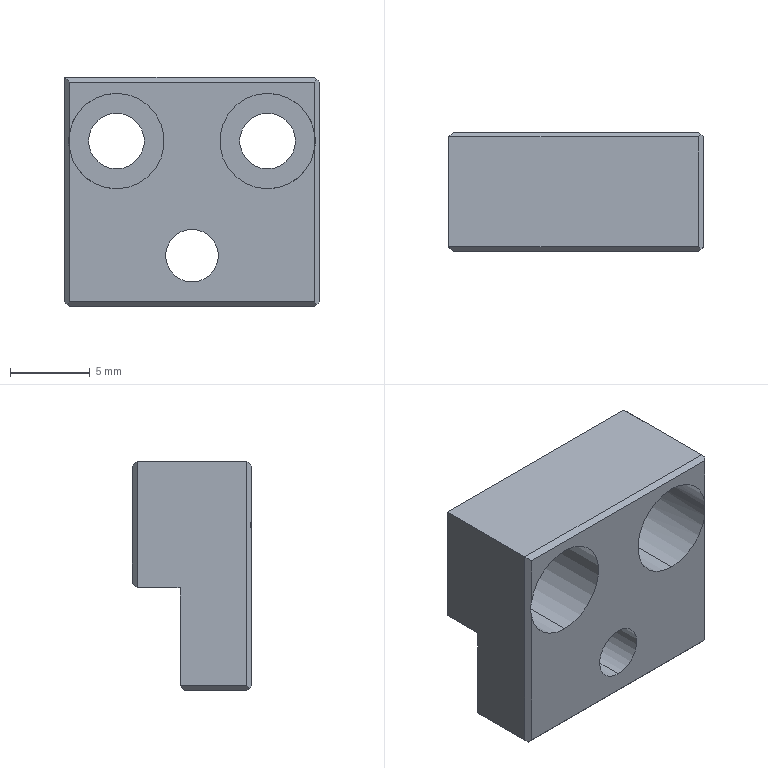Part | NX | 1 solid | 32 faces | box 16 x 7.5 x 14.4 mm | volume 1061 mm3 | plane 22 | cylinder 10 | commonest cylinder face diameters 3.5 x4 6 x4 3.3 x2
STEP:
#1=CARTESIAN_POINT('',(16.39,-63.429,11.453));
#2=VERTEX_POINT('',#1);
#3=CARTESIAN_POINT('',(0.3897,-63.429,11.453));
#4=VERTEX_POINT('',#3);
#5=CARTESIAN_POINT('',(8.39,-63.429,11.453));
#6=DIRECTION('',(-1.,0.,0.));
#7=VECTOR('',#6,1000.);
#8=LINE('',#5,#7);
#9=EDGE_CURVE('',#2,#4,#8,.T.);
#10=ORIENTED_EDGE('',*,*,#9,.F.);
#11=CARTESIAN_POINT('',(16.39,-66.129,11.453));
#12=VERTEX_POINT('',#11);
#13=CARTESIAN_POINT('',(16.39,-59.69,11.453));
#14=DIRECTION('',(0.,1.,0.));
#15=VECTOR('',#14,1000.);
#16=LINE('',#13,#15);
#17=EDGE_CURVE('',#12,#2,#16,.T.);
#18=ORIENTED_EDGE('',*,*,#17,.F.);
#19=CARTESIAN_POINT('',(0.3897,-66.129,11.453));
#20=VERTEX_POINT('',#19);
#21=CARTESIAN_POINT('',(13.89,-66.129,11.453));
#22=DIRECTION('',(-1.,0.,0.));
#23=VECTOR('',#22,1000.);
#24=LINE('',#21,#23);
#25=EDGE_CURVE('',#12,#20,#24,.T.);
#26=ORIENTED_EDGE('',*,*,#25,.T.);
#27=CARTESIAN_POINT('',(0.3897,-59.69,11.453));
#28=DIRECTION('',(0.,1.,0.));
#29=VECTOR('',#28,1000.);
#30=LINE('',#27,#29);
#31=EDGE_CURVE('',#20,#4,#30,.T.);
#32=ORIENTED_EDGE('',*,*,#31,.T.);
#33=EDGE_LOOP('',(#10,#18,#26,#32));
#34=FACE_BOUND('',#33,.T.);
#35=CARTESIAN_POINT('',(13.89,-66.629,11.453));
#36=DIRECTION('',(0.,0.,-1.));
#37=DIRECTION('',(0.,-1.,0.));
#38=AXIS2_PLACEMENT_3D('',#35,#36,#37);
#39=PLANE('',#38);
#40=ADVANCED_FACE('',(#34),#39,.T.);
#41=CARTESIAN_POINT('',(16.39,-66.129,5.303));
#42=VERTEX_POINT('',#41);
#43=CARTESIAN_POINT('',(0.3897,-66.129,5.303));
#44=VERTEX_POINT('',#43);
#45=CARTESIAN_POINT('',(8.39,-66.129,5.303));
#46=DIRECTION('',(-1.,0.,0.));
#47=VECTOR('',#46,1000.);
#48=LINE('',#45,#47);
#49=EDGE_CURVE('',#42,#44,#48,.T.);
#50=ORIENTED_EDGE('',*,*,#49,.T.);
#51=CARTESIAN_POINT('',(0.3897,-66.129,11.106));
#52=DIRECTION('',(0.,0.,-1.));
#53=VECTOR('',#52,1000.);
#54=LINE('',#51,#53);
#55=EDGE_CURVE('',#20,#44,#54,.T.);
#56=ORIENTED_EDGE('',*,*,#55,.F.);
#57=ORIENTED_EDGE('',*,*,#25,.F.);
#58=CARTESIAN_POINT('',(16.39,-66.129,11.106));
#59=DIRECTION('',(0.,0.,-1.));
#60=VECTOR('',#59,1000.);
#61=LINE('',#58,#60);
#62=EDGE_CURVE('',#12,#42,#61,.T.);
#63=ORIENTED_EDGE('',*,*,#62,.T.);
#64=EDGE_LOOP('',(#50,#56,#57,#63));
#65=FACE_BOUND('',#64,.T.);
#66=CARTESIAN_POINT('',(8.39,-66.129,6.553));
#67=VERTEX_POINT('',#66);
#68=CARTESIAN_POINT('',(8.39,-66.129,9.853));
#69=VERTEX_POINT('',#68);
#70=CARTESIAN_POINT('',(8.39,-66.129,8.203));
#71=DIRECTION('',(0.,-1.,0.));
#72=DIRECTION('',(0.,0.,1.));
#73=AXIS2_PLACEMENT_3D('',#70,#71,#72);
#74=CIRCLE('',#73,1.65);
#75=EDGE_CURVE('',#67,#69,#74,.T.);
#76=ORIENTED_EDGE('',*,*,#75,.T.);
#77=CARTESIAN_POINT('',(8.39,-66.129,8.203));
#78=DIRECTION('',(0.,-1.,0.));
#79=DIRECTION('',(0.,0.,1.));
#80=AXIS2_PLACEMENT_3D('',#77,#78,#79);
#81=CIRCLE('',#80,1.65);
#82=EDGE_CURVE('',#69,#67,#81,.T.);
#83=ORIENTED_EDGE('',*,*,#82,.T.);
#84=EDGE_LOOP('',(#76,#83));
#85=FACE_BOUND('',#84,.T.);
#86=CARTESIAN_POINT('',(13.89,-66.129,5.503));
#87=DIRECTION('',(0.,1.,0.));
#88=DIRECTION('',(1.,0.,0.));
#89=AXIS2_PLACEMENT_3D('',#86,#87,#88);
#90=PLANE('',#89);
#91=ADVANCED_FACE('',(#65,#85),#90,.T.);
#92=CARTESIAN_POINT('',(0.6897,-70.329,5.003));
#93=VERTEX_POINT('',#92);
#94=CARTESIAN_POINT('',(16.09,-70.329,5.003));
#95=VERTEX_POINT('',#94);
#96=CARTESIAN_POINT('',(8.39,-70.329,5.003));
#97=DIRECTION('',(1.,0.,0.));
#98=VECTOR('',#97,1000.);
#99=LINE('',#96,#98);
#100=EDGE_CURVE('',#93,#95,#99,.T.);
#101=ORIENTED_EDGE('',*,*,#100,.F.);
#102=CARTESIAN_POINT('',(0.6897,-66.429,5.003));
#103=VERTEX_POINT('',#102);
#104=CARTESIAN_POINT('',(0.6897,-68.379,5.003));
#105=DIRECTION('',(0.,-1.,0.));
#106=VECTOR('',#105,1000.);
#107=LINE('',#104,#106);
#108=EDGE_CURVE('',#103,#93,#107,.T.);
#109=ORIENTED_EDGE('',*,*,#108,.F.);
#110=CARTESIAN_POINT('',(16.09,-66.429,5.003));
#111=VERTEX_POINT('',#110);
#112=CARTESIAN_POINT('',(8.39,-66.429,5.003));
#113=DIRECTION('',(-1.,0.,0.));
#114=VECTOR('',#113,1000.);
#115=LINE('',#112,#114);
#116=EDGE_CURVE('',#111,#103,#115,.T.);
#117=ORIENTED_EDGE('',*,*,#116,.F.);
#118=CARTESIAN_POINT('',(16.09,-68.379,5.003));
#119=DIRECTION('',(0.,-1.,0.));
#120=VECTOR('',#119,1000.);
#121=LINE('',#118,#120);
#122=EDGE_CURVE('',#111,#95,#121,.T.);
#123=ORIENTED_EDGE('',*,*,#122,.T.);
#124=EDGE_LOOP('',(#101,#109,#117,#123));
#125=FACE_BOUND('',#124,.T.);
#126=CARTESIAN_POINT('',(13.89,-70.329,5.003));
#127=DIRECTION('',(0.,0.,-1.));
#128=DIRECTION('',(0.,-1.,0.));
#129=AXIS2_PLACEMENT_3D('',#126,#127,#128);
#130=PLANE('',#129);
#131=ADVANCED_FACE('',(#125),#130,.T.);
#132=CARTESIAN_POINT('',(16.09,-70.629,19.103));
#133=VERTEX_POINT('',#132);
#134=CARTESIAN_POINT('',(0.6897,-70.629,19.103));
#135=VERTEX_POINT('',#134);
#136=CARTESIAN_POINT('',(8.39,-70.629,19.103));
#137=DIRECTION('',(-1.,0.,0.));
#138=VECTOR('',#137,1000.);
#139=LINE('',#136,#138);
#140=EDGE_CURVE('',#133,#135,#139,.T.);
#141=ORIENTED_EDGE('',*,*,#140,.T.);
#142=CARTESIAN_POINT('',(0.6897,-70.629,15.949));
#143=VERTEX_POINT('',#142);
#144=CARTESIAN_POINT('',(0.6897,-70.629,11.106));
#145=DIRECTION('',(0.,0.,-1.));
#146=VECTOR('',#145,1000.);
#147=LINE('',#144,#146);
#148=EDGE_CURVE('',#135,#143,#147,.T.);
#149=ORIENTED_EDGE('',*,*,#148,.T.);
#150=CARTESIAN_POINT('',(3.64,-70.629,18.403));
#151=VERTEX_POINT('',#150);
#152=CARTESIAN_POINT('',(3.64,-70.629,15.403));
#153=DIRECTION('',(0.,-1.,0.));
#154=DIRECTION('',(0.,0.,1.));
#155=AXIS2_PLACEMENT_3D('',#152,#153,#154);
#156=CIRCLE('',#155,3.);
#157=EDGE_CURVE('',#151,#143,#156,.T.);
#158=ORIENTED_EDGE('',*,*,#157,.F.);
#159=CARTESIAN_POINT('',(3.64,-70.629,12.403));
#160=VERTEX_POINT('',#159);
#161=CARTESIAN_POINT('',(3.64,-70.629,15.403));
#162=DIRECTION('',(0.,-1.,0.));
#163=DIRECTION('',(0.,0.,1.));
#164=AXIS2_PLACEMENT_3D('',#161,#162,#163);
#165=CIRCLE('',#164,3.);
#166=EDGE_CURVE('',#160,#151,#165,.T.);
#167=ORIENTED_EDGE('',*,*,#166,.F.);
#168=CARTESIAN_POINT('',(0.6897,-70.629,14.858));
#169=VERTEX_POINT('',#168);
#170=CARTESIAN_POINT('',(3.64,-70.629,15.403));
#171=DIRECTION('',(0.,-1.,0.));
#172=DIRECTION('',(0.,0.,1.));
#173=AXIS2_PLACEMENT_3D('',#170,#171,#172);
#174=CIRCLE('',#173,3.);
#175=EDGE_CURVE('',#169,#160,#174,.T.);
#176=ORIENTED_EDGE('',*,*,#175,.F.);
#177=CARTESIAN_POINT('',(0.6897,-70.629,5.303));
#178=VERTEX_POINT('',#177);
#179=CARTESIAN_POINT('',(0.6897,-70.629,11.106));
#180=DIRECTION('',(0.,0.,-1.));
#181=VECTOR('',#180,1000.);
#182=LINE('',#179,#181);
#183=EDGE_CURVE('',#169,#178,#182,.T.);
#184=ORIENTED_EDGE('',*,*,#183,.T.);
#185=CARTESIAN_POINT('',(16.09,-70.629,5.303));
#186=VERTEX_POINT('',#185);
#187=CARTESIAN_POINT('',(8.39,-70.629,5.303));
#188=DIRECTION('',(1.,0.,0.));
#189=VECTOR('',#188,1000.);
#190=LINE('',#187,#189);
#191=EDGE_CURVE('',#178,#186,#190,.T.);
#192=ORIENTED_EDGE('',*,*,#191,.T.);
#193=CARTESIAN_POINT('',(16.09,-70.629,14.858));
#194=VERTEX_POINT('',#193);
#195=CARTESIAN_POINT('',(16.09,-70.629,11.106));
#196=DIRECTION('',(0.,0.,-1.));
#197=VECTOR('',#196,1000.);
#198=LINE('',#195,#197);
#199=EDGE_CURVE('',#194,#186,#198,.T.);
#200=ORIENTED_EDGE('',*,*,#199,.F.);
#201=CARTESIAN_POINT('',(13.14,-70.629,12.403));
#202=VERTEX_POINT('',#201);
#203=CARTESIAN_POINT('',(13.14,-70.629,15.403));
#204=DIRECTION('',(0.,-1.,0.));
#205=DIRECTION('',(0.,0.,1.));
#206=AXIS2_PLACEMENT_3D('',#203,#204,#205);
#207=CIRCLE('',#206,3.);
#208=EDGE_CURVE('',#202,#194,#207,.T.);
#209=ORIENTED_EDGE('',*,*,#208,.F.);
#210=CARTESIAN_POINT('',(13.14,-70.629,18.403));
#211=VERTEX_POINT('',#210);
#212=CARTESIAN_POINT('',(13.14,-70.629,15.403));
#213=DIRECTION('',(0.,-1.,0.));
#214=DIRECTION('',(0.,0.,1.));
#215=AXIS2_PLACEMENT_3D('',#212,#213,#214);
#216=CIRCLE('',#215,3.);
#217=EDGE_CURVE('',#211,#202,#216,.T.);
#218=ORIENTED_EDGE('',*,*,#217,.F.);
#219=CARTESIAN_POINT('',(16.09,-70.629,15.949));
#220=VERTEX_POINT('',#219);
#221=CARTESIAN_POINT('',(13.14,-70.629,15.403));
#222=DIRECTION('',(0.,-1.,0.));
#223=DIRECTION('',(0.,0.,1.));
#224=AXIS2_PLACEMENT_3D('',#221,#222,#223);
#225=CIRCLE('',#224,3.);
#226=EDGE_CURVE('',#220,#211,#225,.T.);
#227=ORIENTED_EDGE('',*,*,#226,.F.);
#228=CARTESIAN_POINT('',(16.09,-70.629,11.106));
#229=DIRECTION('',(0.,0.,-1.));
#230=VECTOR('',#229,1000.);
#231=LINE('',#228,#230);
#232=EDGE_CURVE('',#133,#220,#231,.T.);
#233=ORIENTED_EDGE('',*,*,#232,.F.);
#234=EDGE_LOOP('',(#141,#149,#158,#167,#176,#184,#192,#200,#209,#218,#227,#233));
#235=FACE_BOUND('',#234,.T.);
#236=CARTESIAN_POINT('',(8.39,-70.629,6.553));
#237=VERTEX_POINT('',#236);
#238=CARTESIAN_POINT('',(8.39,-70.629,9.853));
#239=VERTEX_POINT('',#238);
#240=CARTESIAN_POINT('',(8.39,-70.629,8.203));
#241=DIRECTION('',(0.,-1.,0.));
#242=DIRECTION('',(0.,0.,1.));
#243=AXIS2_PLACEMENT_3D('',#240,#241,#242);
#244=CIRCLE('',#243,1.65);
#245=EDGE_CURVE('',#237,#239,#244,.T.);
#246=ORIENTED_EDGE('',*,*,#245,.F.);
#247=CARTESIAN_POINT('',(8.39,-70.629,8.203));
#248=DIRECTION('',(0.,-1.,0.));
#249=DIRECTION('',(0.,0.,1.));
#250=AXIS2_PLACEMENT_3D('',#247,#248,#249);
#251=CIRCLE('',#250,1.65);
#252=EDGE_CURVE('',#239,#237,#251,.T.);
#253=ORIENTED_EDGE('',*,*,#252,.F.);
#254=EDGE_LOOP('',(#246,#253));
#255=FACE_BOUND('',#254,.T.);
#256=CARTESIAN_POINT('',(13.89,-70.629,20.403));
#257=DIRECTION('',(0.,-1.,0.));
#258=DIRECTION('',(-1.,0.,0.));
#259=AXIS2_PLACEMENT_3D('',#256,#257,#258);
#260=PLANE('',#259);
#261=ADVANCED_FACE('',(#235,#255),#260,.T.);
#262=CARTESIAN_POINT('',(0.3897,-63.429,19.403));
#263=VERTEX_POINT('',#262);
#264=CARTESIAN_POINT('',(16.09,-63.429,19.403));
#265=VERTEX_POINT('',#264);
#266=CARTESIAN_POINT('',(8.39,-63.429,19.403));
#267=DIRECTION('',(1.,0.,0.));
#268=VECTOR('',#267,1000.);
#269=LINE('',#266,#268);
#270=EDGE_CURVE('',#263,#265,#269,.T.);
#271=ORIENTED_EDGE('',*,*,#270,.F.);
#272=CARTESIAN_POINT('',(0.3897,-70.329,19.403));
#273=VERTEX_POINT('',#272);
#274=CARTESIAN_POINT('',(0.3897,-59.69,19.403));
#275=DIRECTION('',(0.,1.,0.));
#276=VECTOR('',#275,1000.);
#277=LINE('',#274,#276);
#278=EDGE_CURVE('',#273,#263,#277,.T.);
#279=ORIENTED_EDGE('',*,*,#278,.F.);
#280=CARTESIAN_POINT('',(16.09,-70.329,19.403));
#281=VERTEX_POINT('',#280);
#282=CARTESIAN_POINT('',(8.39,-70.329,19.403));
#283=DIRECTION('',(-1.,0.,0.));
#284=VECTOR('',#283,1000.);
#285=LINE('',#282,#284);
#286=EDGE_CURVE('',#281,#273,#285,.T.);
#287=ORIENTED_EDGE('',*,*,#286,.F.);
#288=CARTESIAN_POINT('',(16.09,-66.879,19.403));
#289=DIRECTION('',(0.,1.,0.));
#290=VECTOR('',#289,1000.);
#291=LINE('',#288,#290);
#292=EDGE_CURVE('',#281,#265,#291,.T.);
#293=ORIENTED_EDGE('',*,*,#292,.T.);
#294=EDGE_LOOP('',(#271,#279,#287,#293));
#295=FACE_BOUND('',#294,.T.);
#296=CARTESIAN_POINT('',(13.89,-63.129,19.403));
#297=DIRECTION('',(0.,0.,1.));
#298=DIRECTION('',(1.,0.,0.));
#299=AXIS2_PLACEMENT_3D('',#296,#297,#298);
#300=PLANE('',#299);
#301=ADVANCED_FACE('',(#295),#300,.T.);
#302=CARTESIAN_POINT('',(16.09,-63.129,19.103));
#303=VERTEX_POINT('',#302);
#304=CARTESIAN_POINT('',(16.09,-63.129,11.753));
#305=VERTEX_POINT('',#304);
#306=CARTESIAN_POINT('',(16.09,-63.129,15.428));
#307=DIRECTION('',(0.,0.,-1.));
#308=VECTOR('',#307,1000.);
#309=LINE('',#306,#308);
#310=EDGE_CURVE('',#303,#305,#309,.T.);
#311=ORIENTED_EDGE('',*,*,#310,.T.);
#312=CARTESIAN_POINT('',(0.6897,-63.129,11.753));
#313=VERTEX_POINT('',#312);
#314=CARTESIAN_POINT('',(8.39,-63.129,11.753));
#315=DIRECTION('',(-1.,0.,0.));
#316=VECTOR('',#315,1000.);
#317=LINE('',#314,#316);
#318=EDGE_CURVE('',#305,#313,#317,.T.);
#319=ORIENTED_EDGE('',*,*,#318,.T.);
#320=CARTESIAN_POINT('',(0.6897,-63.129,19.103));
#321=VERTEX_POINT('',#320);
#322=CARTESIAN_POINT('',(0.6897,-63.129,15.428));
#323=DIRECTION('',(0.,0.,-1.));
#324=VECTOR('',#323,1000.);
#325=LINE('',#322,#324);
#326=EDGE_CURVE('',#321,#313,#325,.T.);
#327=ORIENTED_EDGE('',*,*,#326,.F.);
#328=CARTESIAN_POINT('',(8.39,-63.129,19.103));
#329=DIRECTION('',(1.,0.,0.));
#330=VECTOR('',#329,1000.);
#331=LINE('',#328,#330);
#332=EDGE_CURVE('',#321,#303,#331,.T.);
#333=ORIENTED_EDGE('',*,*,#332,.T.);
#334=EDGE_LOOP('',(#311,#319,#327,#333));
#335=FACE_BOUND('',#334,.T.);
#336=CARTESIAN_POINT('',(3.64,-63.129,13.653));
#337=VERTEX_POINT('',#336);
#338=CARTESIAN_POINT('',(3.64,-63.129,17.153));
#339=VERTEX_POINT('',#338);
#340=CARTESIAN_POINT('',(3.64,-63.129,15.403));
#341=DIRECTION('',(0.,-1.,0.));
#342=DIRECTION('',(0.,0.,1.));
#343=AXIS2_PLACEMENT_3D('',#340,#341,#342);
#344=CIRCLE('',#343,1.75);
#345=EDGE_CURVE('',#337,#339,#344,.T.);
#346=ORIENTED_EDGE('',*,*,#345,.T.);
#347=CARTESIAN_POINT('',(3.64,-63.129,15.403));
#348=DIRECTION('',(0.,-1.,0.));
#349=DIRECTION('',(0.,0.,1.));
#350=AXIS2_PLACEMENT_3D('',#347,#348,#349);
#351=CIRCLE('',#350,1.75);
#352=EDGE_CURVE('',#339,#337,#351,.T.);
#353=ORIENTED_EDGE('',*,*,#352,.T.);
#354=EDGE_LOOP('',(#346,#353));
#355=FACE_BOUND('',#354,.T.);
#356=CARTESIAN_POINT('',(13.14,-63.129,13.653));
#357=VERTEX_POINT('',#356);
#358=CARTESIAN_POINT('',(13.14,-63.129,17.153));
#359=VERTEX_POINT('',#358);
#360=CARTESIAN_POINT('',(13.14,-63.129,15.403));
#361=DIRECTION('',(0.,-1.,0.));
#362=DIRECTION('',(0.,0.,1.));
#363=AXIS2_PLACEMENT_3D('',#360,#361,#362);
#364=CIRCLE('',#363,1.75);
#365=EDGE_CURVE('',#357,#359,#364,.T.);
#366=ORIENTED_EDGE('',*,*,#365,.T.);
#367=CARTESIAN_POINT('',(13.14,-63.129,15.403));
#368=DIRECTION('',(0.,-1.,0.));
#369=DIRECTION('',(0.,0.,1.));
#370=AXIS2_PLACEMENT_3D('',#367,#368,#369);
#371=CIRCLE('',#370,1.75);
#372=EDGE_CURVE('',#359,#357,#371,.T.);
#373=ORIENTED_EDGE('',*,*,#372,.T.);
#374=EDGE_LOOP('',(#366,#373));
#375=FACE_BOUND('',#374,.T.);
#376=CARTESIAN_POINT('',(13.89,-63.129,11.253));
#377=DIRECTION('',(0.,1.,0.));
#378=DIRECTION('',(1.,0.,0.));
#379=AXIS2_PLACEMENT_3D('',#376,#377,#378);
#380=PLANE('',#379);
#381=ADVANCED_FACE('',(#335,#355,#375),#380,.T.);
#382=ORIENTED_EDGE('',*,*,#157,.T.);
#383=CARTESIAN_POINT('',(0.6897,-70.629,15.949));
#384=CARTESIAN_POINT('',(0.6229,-70.562,15.587));
#385=CARTESIAN_POINT('',(0.6229,-70.562,15.219));
#386=CARTESIAN_POINT('',(0.6897,-70.629,14.858));
#387=(BOUNDED_CURVE()B_SPLINE_CURVE(3,(#383,#384,#385,#386),.UNSPECIFIED.,.F.,.F.)B_SPLINE_CURVE_WITH_KNOTS((4,4),(2.959,3.324),.UNSPECIFIED.)CURVE()GEOMETRIC_REPRESENTATION_ITEM()RATIONAL_B_SPLINE_CURVE((1.,0.9889,0.9889,1.))REPRESENTATION_ITEM(''));
#388=EDGE_CURVE('',#143,#169,#387,.T.);
#389=ORIENTED_EDGE('',*,*,#388,.T.);
#390=ORIENTED_EDGE('',*,*,#175,.T.);
#391=CARTESIAN_POINT('',(3.64,-66.129,12.403));
#392=VERTEX_POINT('',#391);
#393=CARTESIAN_POINT('',(3.64,-69.629,12.403));
#394=DIRECTION('',(0.,-1.,0.));
#395=VECTOR('',#394,1000.);
#396=LINE('',#393,#395);
#397=EDGE_CURVE('',#160,#392,#396,.F.);
#398=ORIENTED_EDGE('',*,*,#397,.T.);
#399=CARTESIAN_POINT('',(3.64,-66.129,18.403));
#400=VERTEX_POINT('',#399);
#401=CARTESIAN_POINT('',(3.64,-66.129,15.403));
#402=DIRECTION('',(0.,-1.,0.));
#403=DIRECTION('',(0.,0.,1.));
#404=AXIS2_PLACEMENT_3D('',#401,#402,#403);
#405=CIRCLE('',#404,3.);
#406=EDGE_CURVE('',#400,#392,#405,.T.);
#407=ORIENTED_EDGE('',*,*,#406,.F.);
#408=CARTESIAN_POINT('',(3.64,-69.629,18.403));
#409=DIRECTION('',(0.,-1.,0.));
#410=VECTOR('',#409,1000.);
#411=LINE('',#408,#410);
#412=EDGE_CURVE('',#151,#400,#411,.F.);
#413=ORIENTED_EDGE('',*,*,#412,.F.);
#414=EDGE_LOOP('',(#382,#389,#390,#398,#407,#413));
#415=FACE_BOUND('',#414,.T.);
#416=CARTESIAN_POINT('',(3.64,-69.629,15.403));
#417=DIRECTION('',(0.,-1.,0.));
#418=DIRECTION('',(0.,0.,1.));
#419=AXIS2_PLACEMENT_3D('',#416,#417,#418);
#420=CYLINDRICAL_SURFACE('',#419,3.);
#421=ADVANCED_FACE('',(#415),#420,.F.);
#422=CARTESIAN_POINT('',(3.64,-66.129,15.403));
#423=DIRECTION('',(0.,-1.,0.));
#424=DIRECTION('',(0.,0.,1.));
#425=AXIS2_PLACEMENT_3D('',#422,#423,#424);
#426=CIRCLE('',#425,3.);
#427=EDGE_CURVE('',#392,#400,#426,.T.);
#428=ORIENTED_EDGE('',*,*,#427,.T.);
#429=ORIENTED_EDGE('',*,*,#406,.T.);
#430=EDGE_LOOP('',(#428,#429));
#431=FACE_BOUND('',#430,.T.);
#432=CARTESIAN_POINT('',(3.64,-66.129,13.653));
#433=VERTEX_POINT('',#432);
#434=CARTESIAN_POINT('',(3.64,-66.129,17.153));
#435=VERTEX_POINT('',#434);
#436=CARTESIAN_POINT('',(3.64,-66.129,15.403));
#437=DIRECTION('',(0.,-1.,0.));
#438=DIRECTION('',(0.,0.,1.));
#439=AXIS2_PLACEMENT_3D('',#436,#437,#438);
#440=CIRCLE('',#439,1.75);
#441=EDGE_CURVE('',#433,#435,#440,.T.);
#442=ORIENTED_EDGE('',*,*,#441,.F.);
#443=CARTESIAN_POINT('',(3.64,-66.129,15.403));
#444=DIRECTION('',(0.,-1.,0.));
#445=DIRECTION('',(0.,0.,1.));
#446=AXIS2_PLACEMENT_3D('',#443,#444,#445);
#447=CIRCLE('',#446,1.75);
#448=EDGE_CURVE('',#435,#433,#447,.T.);
#449=ORIENTED_EDGE('',*,*,#448,.F.);
#450=EDGE_LOOP('',(#442,#449));
#451=FACE_BOUND('',#450,.T.);
#452=CARTESIAN_POINT('',(3.64,-66.129,15.403));
#453=DIRECTION('',(0.,-1.,0.));
#454=DIRECTION('',(-1.,0.,0.));
#455=AXIS2_PLACEMENT_3D('',#452,#453,#454);
#456=PLANE('',#455);
#457=ADVANCED_FACE('',(#431,#451),#456,.T.);
#458=ORIENTED_EDGE('',*,*,#441,.T.);
#459=CARTESIAN_POINT('',(3.64,-69.629,17.153));
#460=DIRECTION('',(0.,-1.,0.));
#461=VECTOR('',#460,1000.);
#462=LINE('',#459,#461);
#463=EDGE_CURVE('',#339,#435,#462,.T.);
#464=ORIENTED_EDGE('',*,*,#463,.F.);
#465=ORIENTED_EDGE('',*,*,#345,.F.);
#466=CARTESIAN_POINT('',(3.64,-69.629,13.653));
#467=DIRECTION('',(0.,-1.,0.));
#468=VECTOR('',#467,1000.);
#469=LINE('',#466,#468);
#470=EDGE_CURVE('',#337,#433,#469,.T.);
#471=ORIENTED_EDGE('',*,*,#470,.T.);
#472=EDGE_LOOP('',(#458,#464,#465,#471));
#473=FACE_BOUND('',#472,.T.);
#474=CARTESIAN_POINT('',(3.64,-69.629,15.403));
#475=DIRECTION('',(0.,-1.,0.));
#476=DIRECTION('',(0.,0.,1.));
#477=AXIS2_PLACEMENT_3D('',#474,#475,#476);
#478=CYLINDRICAL_SURFACE('',#477,1.75);
#479=ADVANCED_FACE('',(#473),#478,.F.);
#480=CARTESIAN_POINT('',(13.14,-66.129,13.653));
#481=VERTEX_POINT('',#480);
#482=CARTESIAN_POINT('',(13.14,-66.129,17.153));
#483=VERTEX_POINT('',#482);
#484=CARTESIAN_POINT('',(13.14,-66.129,15.403));
#485=DIRECTION('',(0.,-1.,0.));
#486=DIRECTION('',(0.,0.,1.));
#487=AXIS2_PLACEMENT_3D('',#484,#485,#486);
#488=CIRCLE('',#487,1.75);
#489=EDGE_CURVE('',#481,#483,#488,.T.);
#490=ORIENTED_EDGE('',*,*,#489,.T.);
#491=CARTESIAN_POINT('',(13.14,-69.629,17.153));
#492=DIRECTION('',(0.,-1.,0.));
#493=VECTOR('',#492,1000.);
#494=LINE('',#491,#493);
#495=EDGE_CURVE('',#483,#359,#494,.F.);
#496=ORIENTED_EDGE('',*,*,#495,.T.);
#497=ORIENTED_EDGE('',*,*,#365,.F.);
#498=CARTESIAN_POINT('',(13.14,-69.629,13.653));
#499=DIRECTION('',(0.,-1.,0.));
#500=VECTOR('',#499,1000.);
#501=LINE('',#498,#500);
#502=EDGE_CURVE('',#481,#357,#501,.F.);
#503=ORIENTED_EDGE('',*,*,#502,.F.);
#504=EDGE_LOOP('',(#490,#496,#497,#503));
#505=FACE_BOUND('',#504,.T.);
#506=CARTESIAN_POINT('',(13.14,-69.629,15.403));
#507=DIRECTION('',(0.,-1.,0.));
#508=DIRECTION('',(0.,0.,1.));
#509=AXIS2_PLACEMENT_3D('',#506,#507,#508);
#510=CYLINDRICAL_SURFACE('',#509,1.75);
#511=ADVANCED_FACE('',(#505),#510,.F.);
#512=CARTESIAN_POINT('',(13.14,-66.129,12.403));
#513=VERTEX_POINT('',#512);
#514=CARTESIAN_POINT('',(13.14,-66.129,18.403));
#515=VERTEX_POINT('',#514);
#516=CARTESIAN_POINT('',(13.14,-66.129,15.403));
#517=DIRECTION('',(0.,-1.,0.));
#518=DIRECTION('',(0.,0.,1.));
#519=AXIS2_PLACEMENT_3D('',#516,#517,#518);
#520=CIRCLE('',#519,3.);
#521=EDGE_CURVE('',#513,#515,#520,.T.);
#522=ORIENTED_EDGE('',*,*,#521,.T.);
#523=CARTESIAN_POINT('',(13.14,-66.129,15.403));
#524=DIRECTION('',(0.,-1.,0.));
#525=DIRECTION('',(0.,0.,1.));
#526=AXIS2_PLACEMENT_3D('',#523,#524,#525);
#527=CIRCLE('',#526,3.);
#528=EDGE_CURVE('',#515,#513,#527,.T.);
#529=ORIENTED_EDGE('',*,*,#528,.T.);
#530=EDGE_LOOP('',(#522,#529));
#531=FACE_BOUND('',#530,.T.);
#532=ORIENTED_EDGE('',*,*,#489,.F.);
#533=CARTESIAN_POINT('',(13.14,-66.129,15.403));
#534=DIRECTION('',(0.,-1.,0.));
#535=DIRECTION('',(0.,0.,1.));
#536=AXIS2_PLACEMENT_3D('',#533,#534,#535);
#537=CIRCLE('',#536,1.75);
#538=EDGE_CURVE('',#483,#481,#537,.T.);
#539=ORIENTED_EDGE('',*,*,#538,.F.);
#540=EDGE_LOOP('',(#532,#539));
#541=FACE_BOUND('',#540,.T.);
#542=CARTESIAN_POINT('',(13.14,-66.129,15.403));
#543=DIRECTION('',(0.,-1.,0.));
#544=DIRECTION('',(-1.,0.,0.));
#545=AXIS2_PLACEMENT_3D('',#542,#543,#544);
#546=PLANE('',#545);
#547=ADVANCED_FACE('',(#531,#541),#546,.T.);
#548=ORIENTED_EDGE('',*,*,#208,.T.);
#549=CARTESIAN_POINT('',(16.09,-70.629,15.949));
#550=CARTESIAN_POINT('',(16.157,-70.562,15.587));
#551=CARTESIAN_POINT('',(16.157,-70.562,15.219));
#552=CARTESIAN_POINT('',(16.09,-70.629,14.858));
#553=(BOUNDED_CURVE()B_SPLINE_CURVE(3,(#549,#550,#551,#552),.UNSPECIFIED.,.F.,.F.)B_SPLINE_CURVE_WITH_KNOTS((4,4),(2.959,3.324),.UNSPECIFIED.)CURVE()GEOMETRIC_REPRESENTATION_ITEM()RATIONAL_B_SPLINE_CURVE((1.,0.9889,0.9889,1.))REPRESENTATION_ITEM(''));
#554=EDGE_CURVE('',#220,#194,#553,.T.);
#555=ORIENTED_EDGE('',*,*,#554,.F.);
#556=ORIENTED_EDGE('',*,*,#226,.T.);
#557=CARTESIAN_POINT('',(13.14,-69.629,18.403));
#558=DIRECTION('',(0.,-1.,0.));
#559=VECTOR('',#558,1000.);
#560=LINE('',#557,#559);
#561=EDGE_CURVE('',#515,#211,#560,.T.);
#562=ORIENTED_EDGE('',*,*,#561,.F.);
#563=ORIENTED_EDGE('',*,*,#521,.F.);
#564=CARTESIAN_POINT('',(13.14,-69.629,12.403));
#565=DIRECTION('',(0.,-1.,0.));
#566=VECTOR('',#565,1000.);
#567=LINE('',#564,#566);
#568=EDGE_CURVE('',#513,#202,#567,.T.);
#569=ORIENTED_EDGE('',*,*,#568,.T.);
#570=EDGE_LOOP('',(#548,#555,#556,#562,#563,#569));
#571=FACE_BOUND('',#570,.T.);
#572=CARTESIAN_POINT('',(13.14,-69.629,15.403));
#573=DIRECTION('',(0.,-1.,0.));
#574=DIRECTION('',(0.,0.,1.));
#575=AXIS2_PLACEMENT_3D('',#572,#573,#574);
#576=CYLINDRICAL_SURFACE('',#575,3.);
#577=ADVANCED_FACE('',(#571),#576,.F.);
#578=ORIENTED_EDGE('',*,*,#245,.T.);
#579=CARTESIAN_POINT('',(8.39,-69.629,9.853));
#580=DIRECTION('',(0.,-1.,0.));
#581=VECTOR('',#580,1000.);
#582=LINE('',#579,#581);
#583=EDGE_CURVE('',#69,#239,#582,.T.);
#584=ORIENTED_EDGE('',*,*,#583,.F.);
#585=ORIENTED_EDGE('',*,*,#75,.F.);
#586=CARTESIAN_POINT('',(8.39,-69.629,6.553));
#587=DIRECTION('',(0.,-1.,0.));
#588=VECTOR('',#587,1000.);
#589=LINE('',#586,#588);
#590=EDGE_CURVE('',#67,#237,#589,.T.);
#591=ORIENTED_EDGE('',*,*,#590,.T.);
#592=EDGE_LOOP('',(#578,#584,#585,#591));
#593=FACE_BOUND('',#592,.T.);
#594=CARTESIAN_POINT('',(8.39,-69.629,8.203));
#595=DIRECTION('',(0.,-1.,0.));
#596=DIRECTION('',(0.,0.,1.));
#597=AXIS2_PLACEMENT_3D('',#594,#595,#596);
#598=CYLINDRICAL_SURFACE('',#597,1.65);
#599=ADVANCED_FACE('',(#593),#598,.F.);
#600=ORIENTED_EDGE('',*,*,#100,.T.);
#601=CARTESIAN_POINT('',(16.24,-70.479,5.153));
#602=VERTEX_POINT('',#601);
#603=CARTESIAN_POINT('',(5.451,-59.69,-5.635));
#604=DIRECTION('',(0.5774,-0.5774,0.5774));
#605=VECTOR('',#604,1000.);
#606=LINE('',#603,#605);
#607=EDGE_CURVE('',#95,#602,#606,.T.);
#608=ORIENTED_EDGE('',*,*,#607,.T.);
#609=CARTESIAN_POINT('',(27.028,-59.69,-5.635));
#610=DIRECTION('',(-0.5774,-0.5774,0.5774));
#611=VECTOR('',#610,1000.);
#612=LINE('',#609,#611);
#613=EDGE_CURVE('',#602,#186,#612,.T.);
#614=ORIENTED_EDGE('',*,*,#613,.T.);
#615=ORIENTED_EDGE('',*,*,#191,.F.);
#616=CARTESIAN_POINT('',(0.5397,-70.479,5.153));
#617=VERTEX_POINT('',#616);
#618=CARTESIAN_POINT('',(13.89,-83.829,18.503));
#619=DIRECTION('',(-0.5774,0.5774,-0.5774));
#620=VECTOR('',#619,1000.);
#621=LINE('',#618,#620);
#622=EDGE_CURVE('',#178,#617,#621,.T.);
#623=ORIENTED_EDGE('',*,*,#622,.T.);
#624=CARTESIAN_POINT('',(11.328,-59.69,-5.635));
#625=DIRECTION('',(0.5774,0.5774,-0.5774));
#626=VECTOR('',#625,1000.);
#627=LINE('',#624,#626);
#628=EDGE_CURVE('',#617,#93,#627,.T.);
#629=ORIENTED_EDGE('',*,*,#628,.T.);
#630=EDGE_LOOP('',(#600,#608,#614,#615,#623,#629));
#631=FACE_BOUND('',#630,.T.);
#632=CARTESIAN_POINT('',(8.39,-70.479,5.153));
#633=DIRECTION('',(0.,0.7071,0.7071));
#634=DIRECTION('',(1.,0.,0.));
#635=AXIS2_PLACEMENT_3D('',#632,#633,#634);
#636=PLANE('',#635);
#637=ADVANCED_FACE('',(#631),#636,.F.);
#638=ORIENTED_EDGE('',*,*,#140,.F.);
#639=CARTESIAN_POINT('',(16.24,-70.479,19.253));
#640=VERTEX_POINT('',#639);
#641=CARTESIAN_POINT('',(27.028,-59.69,30.042));
#642=DIRECTION('',(0.5774,0.5774,0.5774));
#643=VECTOR('',#642,1000.);
#644=LINE('',#641,#643);
#645=EDGE_CURVE('',#133,#640,#644,.T.);
#646=ORIENTED_EDGE('',*,*,#645,.T.);
#647=CARTESIAN_POINT('',(5.451,-59.69,30.042));
#648=DIRECTION('',(0.5774,-0.5774,-0.5774));
#649=VECTOR('',#648,1000.);
#650=LINE('',#647,#649);
#651=EDGE_CURVE('',#281,#640,#650,.T.);
#652=ORIENTED_EDGE('',*,*,#651,.F.);
#653=ORIENTED_EDGE('',*,*,#286,.T.);
#654=CARTESIAN_POINT('',(13.89,-83.829,5.903));
#655=DIRECTION('',(-0.5774,0.5774,0.5774));
#656=VECTOR('',#655,1000.);
#657=LINE('',#654,#656);
#658=EDGE_CURVE('',#135,#273,#657,.T.);
#659=ORIENTED_EDGE('',*,*,#658,.F.);
#660=EDGE_LOOP('',(#638,#646,#652,#653,#659));
#661=FACE_BOUND('',#660,.T.);
#662=CARTESIAN_POINT('',(8.39,-70.479,19.253));
#663=DIRECTION('',(0.,-0.7071,0.7071));
#664=DIRECTION('',(-1.,0.,0.));
#665=AXIS2_PLACEMENT_3D('',#662,#663,#664);
#666=PLANE('',#665);
#667=ADVANCED_FACE('',(#661),#666,.T.);
#668=ORIENTED_EDGE('',*,*,#270,.T.);
#669=CARTESIAN_POINT('',(16.24,-63.279,19.253));
#670=VERTEX_POINT('',#669);
#671=CARTESIAN_POINT('',(13.89,-65.629,21.603));
#672=DIRECTION('',(-0.5774,-0.5774,0.5774));
#673=VECTOR('',#672,1000.);
#674=LINE('',#671,#673);
#675=EDGE_CURVE('',#670,#265,#674,.T.);
#676=ORIENTED_EDGE('',*,*,#675,.F.);
#677=CARTESIAN_POINT('',(13.89,-60.929,16.903));
#678=DIRECTION('',(-0.5774,0.5774,-0.5774));
#679=VECTOR('',#678,1000.);
#680=LINE('',#677,#679);
#681=EDGE_CURVE('',#670,#303,#680,.T.);
#682=ORIENTED_EDGE('',*,*,#681,.T.);
#683=ORIENTED_EDGE('',*,*,#332,.F.);
#684=CARTESIAN_POINT('',(13.89,-49.929,5.903));
#685=DIRECTION('',(0.5774,0.5774,-0.5774));
#686=VECTOR('',#685,1000.);
#687=LINE('',#684,#686);
#688=EDGE_CURVE('',#263,#321,#687,.T.);
#689=ORIENTED_EDGE('',*,*,#688,.F.);
#690=EDGE_LOOP('',(#668,#676,#682,#683,#689));
#691=FACE_BOUND('',#690,.T.);
#692=CARTESIAN_POINT('',(8.39,-63.279,19.253));
#693=DIRECTION('',(0.,-0.7071,-0.7071));
#694=DIRECTION('',(0.,-0.7071,0.7071));
#695=AXIS2_PLACEMENT_3D('',#692,#693,#694);
#696=PLANE('',#695);
#697=ADVANCED_FACE('',(#691),#696,.F.);
#698=ORIENTED_EDGE('',*,*,#9,.T.);
#699=CARTESIAN_POINT('',(13.89,-49.929,24.953));
#700=DIRECTION('',(-0.5774,-0.5774,-0.5774));
#701=VECTOR('',#700,1000.);
#702=LINE('',#699,#701);
#703=EDGE_CURVE('',#313,#4,#702,.T.);
#704=ORIENTED_EDGE('',*,*,#703,.F.);
#705=ORIENTED_EDGE('',*,*,#318,.F.);
#706=CARTESIAN_POINT('',(16.737,-63.776,11.106));
#707=DIRECTION('',(-0.5774,0.5774,0.5774));
#708=VECTOR('',#707,1000.);
#709=LINE('',#706,#708);
#710=EDGE_CURVE('',#2,#305,#709,.T.);
#711=ORIENTED_EDGE('',*,*,#710,.F.);
#712=EDGE_LOOP('',(#698,#704,#705,#711));
#713=FACE_BOUND('',#712,.T.);
#714=CARTESIAN_POINT('',(8.39,-63.279,11.603));
#715=DIRECTION('',(0.,-0.7071,0.7071));
#716=DIRECTION('',(-1.,0.,0.));
#717=AXIS2_PLACEMENT_3D('',#714,#715,#716);
#718=PLANE('',#717);
#719=ADVANCED_FACE('',(#713),#718,.F.);
#720=ORIENTED_EDGE('',*,*,#49,.F.);
#721=CARTESIAN_POINT('',(13.89,-68.629,2.803));
#722=DIRECTION('',(-0.5774,-0.5774,-0.5774));
#723=VECTOR('',#722,1000.);
#724=LINE('',#721,#723);
#725=EDGE_CURVE('',#42,#111,#724,.T.);
#726=ORIENTED_EDGE('',*,*,#725,.T.);
#727=ORIENTED_EDGE('',*,*,#116,.T.);
#728=CARTESIAN_POINT('',(13.89,-79.629,-8.197));
#729=DIRECTION('',(0.5774,-0.5774,-0.5774));
#730=VECTOR('',#729,1000.);
#731=LINE('',#728,#730);
#732=EDGE_CURVE('',#44,#103,#731,.T.);
#733=ORIENTED_EDGE('',*,*,#732,.F.);
#734=EDGE_LOOP('',(#720,#726,#727,#733));
#735=FACE_BOUND('',#734,.T.);
#736=CARTESIAN_POINT('',(8.39,-66.279,5.153));
#737=DIRECTION('',(0.,0.7071,-0.7071));
#738=DIRECTION('',(-1.,0.,0.));
#739=AXIS2_PLACEMENT_3D('',#736,#737,#738);
#740=PLANE('',#739);
#741=ADVANCED_FACE('',(#735),#740,.T.);
#742=ORIENTED_EDGE('',*,*,#502,.T.);
#743=ORIENTED_EDGE('',*,*,#372,.F.);
#744=ORIENTED_EDGE('',*,*,#495,.F.);
#745=ORIENTED_EDGE('',*,*,#538,.T.);
#746=EDGE_LOOP('',(#742,#743,#744,#745));
#747=FACE_BOUND('',#746,.T.);
#748=CARTESIAN_POINT('',(13.14,-69.629,15.403));
#749=DIRECTION('',(0.,-1.,0.));
#750=DIRECTION('',(0.,0.,1.));
#751=AXIS2_PLACEMENT_3D('',#748,#749,#750);
#752=CYLINDRICAL_SURFACE('',#751,1.75);
#753=ADVANCED_FACE('',(#747),#752,.F.);
#754=ORIENTED_EDGE('',*,*,#427,.F.);
#755=ORIENTED_EDGE('',*,*,#397,.F.);
#756=ORIENTED_EDGE('',*,*,#166,.T.);
#757=ORIENTED_EDGE('',*,*,#412,.T.);
#758=EDGE_LOOP('',(#754,#755,#756,#757));
#759=FACE_BOUND('',#758,.T.);
#760=CARTESIAN_POINT('',(3.64,-69.629,15.403));
#761=DIRECTION('',(0.,-1.,0.));
#762=DIRECTION('',(0.,0.,1.));
#763=AXIS2_PLACEMENT_3D('',#760,#761,#762);
#764=CYLINDRICAL_SURFACE('',#763,3.);
#765=ADVANCED_FACE('',(#759),#764,.F.);
#766=ORIENTED_EDGE('',*,*,#463,.T.);
#767=ORIENTED_EDGE('',*,*,#448,.T.);
#768=ORIENTED_EDGE('',*,*,#470,.F.);
#769=ORIENTED_EDGE('',*,*,#352,.F.);
#770=EDGE_LOOP('',(#766,#767,#768,#769));
#771=FACE_BOUND('',#770,.T.);
#772=CARTESIAN_POINT('',(3.64,-69.629,15.403));
#773=DIRECTION('',(0.,-1.,0.));
#774=DIRECTION('',(0.,0.,1.));
#775=AXIS2_PLACEMENT_3D('',#772,#773,#774);
#776=CYLINDRICAL_SURFACE('',#775,1.75);
#777=ADVANCED_FACE('',(#771),#776,.F.);
#778=ORIENTED_EDGE('',*,*,#583,.T.);
#779=ORIENTED_EDGE('',*,*,#252,.T.);
#780=ORIENTED_EDGE('',*,*,#590,.F.);
#781=ORIENTED_EDGE('',*,*,#82,.F.);
#782=EDGE_LOOP('',(#778,#779,#780,#781));
#783=FACE_BOUND('',#782,.T.);
#784=CARTESIAN_POINT('',(8.39,-69.629,8.203));
#785=DIRECTION('',(0.,-1.,0.));
#786=DIRECTION('',(0.,0.,1.));
#787=AXIS2_PLACEMENT_3D('',#784,#785,#786);
#788=CYLINDRICAL_SURFACE('',#787,1.65);
#789=ADVANCED_FACE('',(#783),#788,.F.);
#790=ORIENTED_EDGE('',*,*,#561,.T.);
#791=ORIENTED_EDGE('',*,*,#217,.T.);
#792=ORIENTED_EDGE('',*,*,#568,.F.);
#793=ORIENTED_EDGE('',*,*,#528,.F.);
#794=EDGE_LOOP('',(#790,#791,#792,#793));
#795=FACE_BOUND('',#794,.T.);
#796=CARTESIAN_POINT('',(13.14,-69.629,15.403));
#797=DIRECTION('',(0.,-1.,0.));
#798=DIRECTION('',(0.,0.,1.));
#799=AXIS2_PLACEMENT_3D('',#796,#797,#798);
#800=CYLINDRICAL_SURFACE('',#799,3.);
#801=ADVANCED_FACE('',(#795),#800,.F.);
#802=CARTESIAN_POINT('',(0.3897,-63.429,15.428));
#803=DIRECTION('',(0.,0.,-1.));
#804=VECTOR('',#803,1000.);
#805=LINE('',#802,#804);
#806=EDGE_CURVE('',#263,#4,#805,.T.);
#807=ORIENTED_EDGE('',*,*,#806,.T.);
#808=ORIENTED_EDGE('',*,*,#31,.F.);
#809=ORIENTED_EDGE('',*,*,#55,.T.);
#810=CARTESIAN_POINT('',(0.3897,-70.329,5.303));
#811=VERTEX_POINT('',#810);
#812=CARTESIAN_POINT('',(0.3897,-68.379,5.303));
#813=DIRECTION('',(0.,-1.,0.));
#814=VECTOR('',#813,1000.);
#815=LINE('',#812,#814);
#816=EDGE_CURVE('',#44,#811,#815,.T.);
#817=ORIENTED_EDGE('',*,*,#816,.T.);
#818=CARTESIAN_POINT('',(0.3897,-70.329,12.203));
#819=DIRECTION('',(0.,0.,1.));
#820=VECTOR('',#819,1000.);
#821=LINE('',#818,#820);
#822=EDGE_CURVE('',#811,#273,#821,.T.);
#823=ORIENTED_EDGE('',*,*,#822,.T.);
#824=ORIENTED_EDGE('',*,*,#278,.T.);
#825=EDGE_LOOP('',(#807,#808,#809,#817,#823,#824));
#826=FACE_BOUND('',#825,.T.);
#827=CARTESIAN_POINT('',(0.3897,-59.69,11.106));
#828=DIRECTION('',(1.,0.,0.));
#829=DIRECTION('',(0.,-1.,0.));
#830=AXIS2_PLACEMENT_3D('',#827,#828,#829);
#831=PLANE('',#830);
#832=ADVANCED_FACE('',(#826),#831,.F.);
#833=ORIENTED_EDGE('',*,*,#822,.F.);
#834=CARTESIAN_POINT('',(13.89,-83.829,-8.197));
#835=DIRECTION('',(0.5774,-0.5774,-0.5774));
#836=VECTOR('',#835,1000.);
#837=LINE('',#834,#836);
#838=EDGE_CURVE('',#811,#617,#837,.T.);
#839=ORIENTED_EDGE('',*,*,#838,.T.);
#840=ORIENTED_EDGE('',*,*,#622,.F.);
#841=ORIENTED_EDGE('',*,*,#183,.F.);
#842=ORIENTED_EDGE('',*,*,#388,.F.);
#843=ORIENTED_EDGE('',*,*,#148,.F.);
#844=ORIENTED_EDGE('',*,*,#658,.T.);
#845=EDGE_LOOP('',(#833,#839,#840,#841,#842,#843,#844));
#846=FACE_BOUND('',#845,.T.);
#847=CARTESIAN_POINT('',(0.5397,-70.479,12.203));
#848=DIRECTION('',(-0.7071,-0.7071,0.));
#849=DIRECTION('',(-0.7071,0.7071,0.));
#850=AXIS2_PLACEMENT_3D('',#847,#848,#849);
#851=PLANE('',#850);
#852=ADVANCED_FACE('',(#846),#851,.T.);
#853=ORIENTED_EDGE('',*,*,#816,.F.);
#854=ORIENTED_EDGE('',*,*,#732,.T.);
#855=ORIENTED_EDGE('',*,*,#108,.T.);
#856=ORIENTED_EDGE('',*,*,#628,.F.);
#857=ORIENTED_EDGE('',*,*,#838,.F.);
#858=EDGE_LOOP('',(#853,#854,#855,#856,#857));
#859=FACE_BOUND('',#858,.T.);
#860=CARTESIAN_POINT('',(0.5397,-68.379,5.153));
#861=DIRECTION('',(-0.7071,0.,-0.7071));
#862=DIRECTION('',(-0.7071,0.,0.7071));
#863=AXIS2_PLACEMENT_3D('',#860,#861,#862);
#864=PLANE('',#863);
#865=ADVANCED_FACE('',(#859),#864,.T.);
#866=ORIENTED_EDGE('',*,*,#806,.F.);
#867=ORIENTED_EDGE('',*,*,#688,.T.);
#868=ORIENTED_EDGE('',*,*,#326,.T.);
#869=ORIENTED_EDGE('',*,*,#703,.T.);
#870=EDGE_LOOP('',(#866,#867,#868,#869));
#871=FACE_BOUND('',#870,.T.);
#872=CARTESIAN_POINT('',(0.5397,-63.279,15.428));
#873=DIRECTION('',(-0.7071,0.7071,0.));
#874=DIRECTION('',(0.,0.,1.));
#875=AXIS2_PLACEMENT_3D('',#872,#873,#874);
#876=PLANE('',#875);
#877=ADVANCED_FACE('',(#871),#876,.T.);
#878=CARTESIAN_POINT('',(16.39,-63.429,19.103));
#879=VERTEX_POINT('',#878);
#880=CARTESIAN_POINT('',(16.39,-63.429,15.428));
#881=DIRECTION('',(0.,0.,-1.));
#882=VECTOR('',#881,1000.);
#883=LINE('',#880,#882);
#884=EDGE_CURVE('',#879,#2,#883,.T.);
#885=ORIENTED_EDGE('',*,*,#884,.F.);
#886=CARTESIAN_POINT('',(16.39,-70.329,19.103));
#887=VERTEX_POINT('',#886);
#888=CARTESIAN_POINT('',(16.39,-66.879,19.103));
#889=DIRECTION('',(0.,1.,0.));
#890=VECTOR('',#889,1000.);
#891=LINE('',#888,#890);
#892=EDGE_CURVE('',#887,#879,#891,.T.);
#893=ORIENTED_EDGE('',*,*,#892,.F.);
#894=CARTESIAN_POINT('',(16.39,-70.329,5.303));
#895=VERTEX_POINT('',#894);
#896=CARTESIAN_POINT('',(16.39,-70.329,12.203));
#897=DIRECTION('',(0.,0.,1.));
#898=VECTOR('',#897,1000.);
#899=LINE('',#896,#898);
#900=EDGE_CURVE('',#895,#887,#899,.T.);
#901=ORIENTED_EDGE('',*,*,#900,.F.);
#902=CARTESIAN_POINT('',(16.39,-68.379,5.303));
#903=DIRECTION('',(0.,-1.,0.));
#904=VECTOR('',#903,1000.);
#905=LINE('',#902,#904);
#906=EDGE_CURVE('',#42,#895,#905,.T.);
#907=ORIENTED_EDGE('',*,*,#906,.F.);
#908=ORIENTED_EDGE('',*,*,#62,.F.);
#909=ORIENTED_EDGE('',*,*,#17,.T.);
#910=EDGE_LOOP('',(#885,#893,#901,#907,#908,#909));
#911=FACE_BOUND('',#910,.T.);
#912=CARTESIAN_POINT('',(16.39,-59.69,11.106));
#913=DIRECTION('',(1.,0.,0.));
#914=DIRECTION('',(0.,-1.,0.));
#915=AXIS2_PLACEMENT_3D('',#912,#913,#914);
#916=PLANE('',#915);
#917=ADVANCED_FACE('',(#911),#916,.T.);
#918=ORIENTED_EDGE('',*,*,#906,.T.);
#919=CARTESIAN_POINT('',(27.028,-59.69,15.942));
#920=DIRECTION('',(-0.5774,-0.5774,-0.5774));
#921=VECTOR('',#920,1000.);
#922=LINE('',#919,#921);
#923=EDGE_CURVE('',#895,#602,#922,.T.);
#924=ORIENTED_EDGE('',*,*,#923,.T.);
#925=ORIENTED_EDGE('',*,*,#607,.F.);
#926=ORIENTED_EDGE('',*,*,#122,.F.);
#927=ORIENTED_EDGE('',*,*,#725,.F.);
#928=EDGE_LOOP('',(#918,#924,#925,#926,#927));
#929=FACE_BOUND('',#928,.T.);
#930=CARTESIAN_POINT('',(16.24,-68.379,5.153));
#931=DIRECTION('',(-0.7071,0.,0.7071));
#932=DIRECTION('',(0.,1.,0.));
#933=AXIS2_PLACEMENT_3D('',#930,#931,#932);
#934=PLANE('',#933);
#935=ADVANCED_FACE('',(#929),#934,.F.);
#936=ORIENTED_EDGE('',*,*,#900,.T.);
#937=CARTESIAN_POINT('',(27.028,-59.69,8.465));
#938=DIRECTION('',(-0.5774,-0.5774,0.5774));
#939=VECTOR('',#938,1000.);
#940=LINE('',#937,#939);
#941=EDGE_CURVE('',#887,#640,#940,.T.);
#942=ORIENTED_EDGE('',*,*,#941,.T.);
#943=ORIENTED_EDGE('',*,*,#645,.F.);
#944=ORIENTED_EDGE('',*,*,#232,.T.);
#945=ORIENTED_EDGE('',*,*,#554,.T.);
#946=ORIENTED_EDGE('',*,*,#199,.T.);
#947=ORIENTED_EDGE('',*,*,#613,.F.);
#948=ORIENTED_EDGE('',*,*,#923,.F.);
#949=EDGE_LOOP('',(#936,#942,#943,#944,#945,#946,#947,#948));
#950=FACE_BOUND('',#949,.T.);
#951=CARTESIAN_POINT('',(16.24,-70.479,12.203));
#952=DIRECTION('',(-0.7071,0.7071,0.));
#953=DIRECTION('',(0.,0.,1.));
#954=AXIS2_PLACEMENT_3D('',#951,#952,#953);
#955=PLANE('',#954);
#956=ADVANCED_FACE('',(#950),#955,.F.);
#957=ORIENTED_EDGE('',*,*,#892,.T.);
#958=CARTESIAN_POINT('',(13.89,-60.929,21.603));
#959=DIRECTION('',(-0.5774,0.5774,0.5774));
#960=VECTOR('',#959,1000.);
#961=LINE('',#958,#960);
#962=EDGE_CURVE('',#879,#670,#961,.T.);
#963=ORIENTED_EDGE('',*,*,#962,.T.);
#964=ORIENTED_EDGE('',*,*,#675,.T.);
#965=ORIENTED_EDGE('',*,*,#292,.F.);
#966=ORIENTED_EDGE('',*,*,#651,.T.);
#967=ORIENTED_EDGE('',*,*,#941,.F.);
#968=EDGE_LOOP('',(#957,#963,#964,#965,#966,#967));
#969=FACE_BOUND('',#968,.T.);
#970=CARTESIAN_POINT('',(16.24,-66.879,19.253));
#971=DIRECTION('',(-0.7071,0.,-0.7071));
#972=DIRECTION('',(-0.7071,0.,0.7071));
#973=AXIS2_PLACEMENT_3D('',#970,#971,#972);
#974=PLANE('',#973);
#975=ADVANCED_FACE('',(#969),#974,.F.);
#976=ORIENTED_EDGE('',*,*,#884,.T.);
#977=ORIENTED_EDGE('',*,*,#710,.T.);
#978=ORIENTED_EDGE('',*,*,#310,.F.);
#979=ORIENTED_EDGE('',*,*,#681,.F.);
#980=ORIENTED_EDGE('',*,*,#962,.F.);
#981=EDGE_LOOP('',(#976,#977,#978,#979,#980));
#982=FACE_BOUND('',#981,.T.);
#983=CARTESIAN_POINT('',(16.24,-63.279,15.428));
#984=DIRECTION('',(-0.7071,-0.7071,0.));
#985=DIRECTION('',(-0.7071,0.7071,0.));
#986=AXIS2_PLACEMENT_3D('',#983,#984,#985);
#987=PLANE('',#986);
#988=ADVANCED_FACE('',(#982),#987,.F.);
#989=CLOSED_SHELL('',(#40,#91,#131,#261,#301,#381,#421,#457,#479,#511,#547,#577,#599,#637,#667,#697,#719,#741,#753,#765,#777,#789,#801,#832,#852,#865,#877,#917,#935,#956,#975,#988));
#990=MANIFOLD_SOLID_BREP('',#989);
#991=(LENGTH_UNIT()NAMED_UNIT(*)SI_UNIT(.MILLI.,.METRE.));
#992=UNCERTAINTY_MEASURE_WITH_UNIT(LENGTH_MEASURE(0.00001),#991,'','');
#993=(NAMED_UNIT(*)PLANE_ANGLE_UNIT()SI_UNIT($,.RADIAN.));
#994=(NAMED_UNIT(*)SI_UNIT($,.STERADIAN.)SOLID_ANGLE_UNIT());
#995=(GEOMETRIC_REPRESENTATION_CONTEXT(3)GLOBAL_UNCERTAINTY_ASSIGNED_CONTEXT((#992))GLOBAL_UNIT_ASSIGNED_CONTEXT((#991,#993,#994))REPRESENTATION_CONTEXT('',''));
#996=ADVANCED_BREP_SHAPE_REPRESENTATION('',(#990),#995);